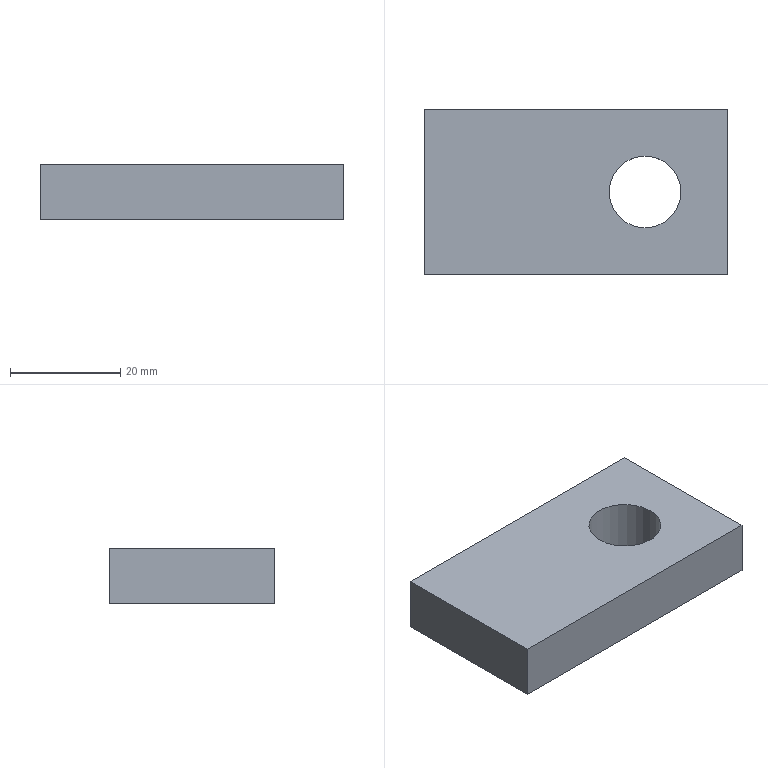Part | NX | features solid 2 | 1 solid | 7 faces | box 55 x 30 x 10 mm | volume 15173 mm3 | plane 6 | cylinder 1 | commonest cylinder face diameters 13 x1
STEP:
#1=CARTESIAN_POINT('',(663.5,75.,-75.));
#2=VERTEX_POINT('',#1);
#3=CARTESIAN_POINT('',(670.,75.,-75.));
#4=DIRECTION('',(0.,0.,-1.));
#5=DIRECTION('',(-1.,0.,0.));
#6=AXIS2_PLACEMENT_3D('',#3,#4,#5);
#7=CIRCLE('',#6,6.5);
#8=EDGE_CURVE('',#2,#2,#7,.F.);
#9=ORIENTED_EDGE('',*,*,#8,.T.);
#10=EDGE_LOOP('',(#9));
#11=FACE_BOUND('',#10,.T.);
#12=CARTESIAN_POINT('',(630.,60.,-75.));
#13=VERTEX_POINT('',#12);
#14=CARTESIAN_POINT('',(630.,90.,-75.));
#15=VERTEX_POINT('',#14);
#16=CARTESIAN_POINT('',(630.,225.,-75.));
#17=DIRECTION('',(0.,-1.,0.));
#18=VECTOR('',#17,1000.);
#19=LINE('',#16,#18);
#20=EDGE_CURVE('',#13,#15,#19,.F.);
#21=ORIENTED_EDGE('',*,*,#20,.T.);
#22=CARTESIAN_POINT('',(685.,90.,-75.));
#23=VERTEX_POINT('',#22);
#24=CARTESIAN_POINT('',(585.,90.,-75.));
#25=DIRECTION('',(-1.,0.,0.));
#26=VECTOR('',#25,1000.);
#27=LINE('',#24,#26);
#28=EDGE_CURVE('',#15,#23,#27,.F.);
#29=ORIENTED_EDGE('',*,*,#28,.T.);
#30=CARTESIAN_POINT('',(685.,60.,-75.));
#31=VERTEX_POINT('',#30);
#32=CARTESIAN_POINT('',(685.,205.,-75.));
#33=DIRECTION('',(0.,1.,0.));
#34=VECTOR('',#33,1000.);
#35=LINE('',#32,#34);
#36=EDGE_CURVE('',#23,#31,#35,.F.);
#37=ORIENTED_EDGE('',*,*,#36,.T.);
#38=CARTESIAN_POINT('',(585.,60.,-75.));
#39=DIRECTION('',(-1.,0.,0.));
#40=VECTOR('',#39,1000.);
#41=LINE('',#38,#40);
#42=EDGE_CURVE('',#13,#31,#41,.F.);
#43=ORIENTED_EDGE('',*,*,#42,.F.);
#44=EDGE_LOOP('',(#21,#29,#37,#43));
#45=FACE_BOUND('',#44,.T.);
#46=CARTESIAN_POINT('',(585.,225.,-75.));
#47=DIRECTION('',(0.,0.,-1.));
#48=DIRECTION('',(0.,1.,0.));
#49=AXIS2_PLACEMENT_3D('',#46,#47,#48);
#50=PLANE('',#49);
#51=ADVANCED_FACE('',(#11,#45),#50,.T.);
#52=CARTESIAN_POINT('',(663.5,75.,-65.));
#53=VERTEX_POINT('',#52);
#54=CARTESIAN_POINT('',(670.,75.,-65.));
#55=DIRECTION('',(0.,0.,-1.));
#56=DIRECTION('',(-1.,0.,0.));
#57=AXIS2_PLACEMENT_3D('',#54,#55,#56);
#58=CIRCLE('',#57,6.5);
#59=EDGE_CURVE('',#53,#53,#58,.T.);
#60=ORIENTED_EDGE('',*,*,#59,.T.);
#61=EDGE_LOOP('',(#60));
#62=FACE_BOUND('',#61,.T.);
#63=CARTESIAN_POINT('',(685.,90.,-65.));
#64=VERTEX_POINT('',#63);
#65=CARTESIAN_POINT('',(630.,90.,-65.));
#66=VERTEX_POINT('',#65);
#67=CARTESIAN_POINT('',(585.,90.,-65.));
#68=DIRECTION('',(-1.,0.,0.));
#69=VECTOR('',#68,1000.);
#70=LINE('',#67,#69);
#71=EDGE_CURVE('',#64,#66,#70,.T.);
#72=ORIENTED_EDGE('',*,*,#71,.T.);
#73=CARTESIAN_POINT('',(630.,60.,-65.));
#74=VERTEX_POINT('',#73);
#75=CARTESIAN_POINT('',(630.,225.,-65.));
#76=DIRECTION('',(0.,1.,0.));
#77=VECTOR('',#76,1000.);
#78=LINE('',#75,#77);
#79=EDGE_CURVE('',#74,#66,#78,.T.);
#80=ORIENTED_EDGE('',*,*,#79,.F.);
#81=CARTESIAN_POINT('',(685.,60.,-65.));
#82=VERTEX_POINT('',#81);
#83=CARTESIAN_POINT('',(585.,60.,-65.));
#84=DIRECTION('',(-1.,0.,0.));
#85=VECTOR('',#84,1000.);
#86=LINE('',#83,#85);
#87=EDGE_CURVE('',#82,#74,#86,.T.);
#88=ORIENTED_EDGE('',*,*,#87,.F.);
#89=CARTESIAN_POINT('',(685.,90.,-65.));
#90=DIRECTION('',(0.,1.,0.));
#91=VECTOR('',#90,1000.);
#92=LINE('',#89,#91);
#93=EDGE_CURVE('',#64,#82,#92,.F.);
#94=ORIENTED_EDGE('',*,*,#93,.F.);
#95=EDGE_LOOP('',(#72,#80,#88,#94));
#96=FACE_BOUND('',#95,.T.);
#97=CARTESIAN_POINT('',(585.,225.,-65.));
#98=DIRECTION('',(0.,0.,-1.));
#99=DIRECTION('',(0.,1.,0.));
#100=AXIS2_PLACEMENT_3D('',#97,#98,#99);
#101=PLANE('',#100);
#102=ADVANCED_FACE('',(#62,#96),#101,.F.);
#103=CARTESIAN_POINT('',(630.,90.,-75.));
#104=DIRECTION('',(0.,0.,1.));
#105=VECTOR('',#104,1000.);
#106=LINE('',#103,#105);
#107=EDGE_CURVE('',#15,#66,#106,.T.);
#108=ORIENTED_EDGE('',*,*,#107,.F.);
#109=ORIENTED_EDGE('',*,*,#20,.F.);
#110=CARTESIAN_POINT('',(630.,60.,-75.));
#111=DIRECTION('',(0.,0.,-1.));
#112=VECTOR('',#111,1000.);
#113=LINE('',#110,#112);
#114=EDGE_CURVE('',#74,#13,#113,.T.);
#115=ORIENTED_EDGE('',*,*,#114,.F.);
#116=ORIENTED_EDGE('',*,*,#79,.T.);
#117=EDGE_LOOP('',(#108,#109,#115,#116));
#118=FACE_BOUND('',#117,.T.);
#119=CARTESIAN_POINT('',(630.,225.,-75.));
#120=DIRECTION('',(1.,0.,0.));
#121=DIRECTION('',(0.,0.,-1.));
#122=AXIS2_PLACEMENT_3D('',#119,#120,#121);
#123=PLANE('',#122);
#124=ADVANCED_FACE('',(#118),#123,.F.);
#125=CARTESIAN_POINT('',(685.,60.,-10.));
#126=DIRECTION('',(0.,0.,-1.));
#127=VECTOR('',#126,1000.);
#128=LINE('',#125,#127);
#129=EDGE_CURVE('',#31,#82,#128,.F.);
#130=ORIENTED_EDGE('',*,*,#129,.F.);
#131=ORIENTED_EDGE('',*,*,#36,.F.);
#132=CARTESIAN_POINT('',(685.,90.,-10.));
#133=DIRECTION('',(0.,0.,1.));
#134=VECTOR('',#133,1000.);
#135=LINE('',#132,#134);
#136=EDGE_CURVE('',#64,#23,#135,.F.);
#137=ORIENTED_EDGE('',*,*,#136,.F.);
#138=ORIENTED_EDGE('',*,*,#93,.T.);
#139=EDGE_LOOP('',(#130,#131,#137,#138));
#140=FACE_BOUND('',#139,.T.);
#141=CARTESIAN_POINT('',(685.,205.,-10.));
#142=DIRECTION('',(1.,0.,0.));
#143=DIRECTION('',(0.,0.,-1.));
#144=AXIS2_PLACEMENT_3D('',#141,#142,#143);
#145=PLANE('',#144);
#146=ADVANCED_FACE('',(#140),#145,.T.);
#147=ORIENTED_EDGE('',*,*,#28,.F.);
#148=ORIENTED_EDGE('',*,*,#107,.T.);
#149=ORIENTED_EDGE('',*,*,#71,.F.);
#150=ORIENTED_EDGE('',*,*,#136,.T.);
#151=EDGE_LOOP('',(#147,#148,#149,#150));
#152=FACE_BOUND('',#151,.T.);
#153=CARTESIAN_POINT('',(670.,90.,-10.));
#154=DIRECTION('',(0.,-1.,0.));
#155=DIRECTION('',(0.,0.,-1.));
#156=AXIS2_PLACEMENT_3D('',#153,#154,#155);
#157=PLANE('',#156);
#158=ADVANCED_FACE('',(#152),#157,.F.);
#159=ORIENTED_EDGE('',*,*,#42,.T.);
#160=ORIENTED_EDGE('',*,*,#129,.T.);
#161=ORIENTED_EDGE('',*,*,#87,.T.);
#162=ORIENTED_EDGE('',*,*,#114,.T.);
#163=EDGE_LOOP('',(#159,#160,#161,#162));
#164=FACE_BOUND('',#163,.T.);
#165=CARTESIAN_POINT('',(670.,60.,-10.));
#166=DIRECTION('',(0.,-1.,0.));
#167=DIRECTION('',(0.,0.,-1.));
#168=AXIS2_PLACEMENT_3D('',#165,#166,#167);
#169=PLANE('',#168);
#170=ADVANCED_FACE('',(#164),#169,.T.);
#171=ORIENTED_EDGE('',*,*,#59,.F.);
#172=EDGE_LOOP('',(#171));
#173=FACE_BOUND('',#172,.T.);
#174=ORIENTED_EDGE('',*,*,#8,.F.);
#175=EDGE_LOOP('',(#174));
#176=FACE_BOUND('',#175,.T.);
#177=CARTESIAN_POINT('',(670.,75.,-65.));
#178=DIRECTION('',(0.,0.,-1.));
#179=DIRECTION('',(-1.,0.,0.));
#180=AXIS2_PLACEMENT_3D('',#177,#178,#179);
#181=CYLINDRICAL_SURFACE('',#180,6.5);
#182=ADVANCED_FACE('',(#173,#176),#181,.F.);
#183=CLOSED_SHELL('',(#51,#102,#124,#146,#158,#170,#182));
#184=MANIFOLD_SOLID_BREP('',#183);
#185=(LENGTH_UNIT()NAMED_UNIT(*)SI_UNIT(.MILLI.,.METRE.));
#186=UNCERTAINTY_MEASURE_WITH_UNIT(LENGTH_MEASURE(0.00001),#185,'','');
#187=(NAMED_UNIT(*)PLANE_ANGLE_UNIT()SI_UNIT($,.RADIAN.));
#188=(NAMED_UNIT(*)SI_UNIT($,.STERADIAN.)SOLID_ANGLE_UNIT());
#189=(GEOMETRIC_REPRESENTATION_CONTEXT(3)GLOBAL_UNCERTAINTY_ASSIGNED_CONTEXT((#186))GLOBAL_UNIT_ASSIGNED_CONTEXT((#185,#187,#188))REPRESENTATION_CONTEXT('',''));
#190=ADVANCED_BREP_SHAPE_REPRESENTATION('',(#184),#189);